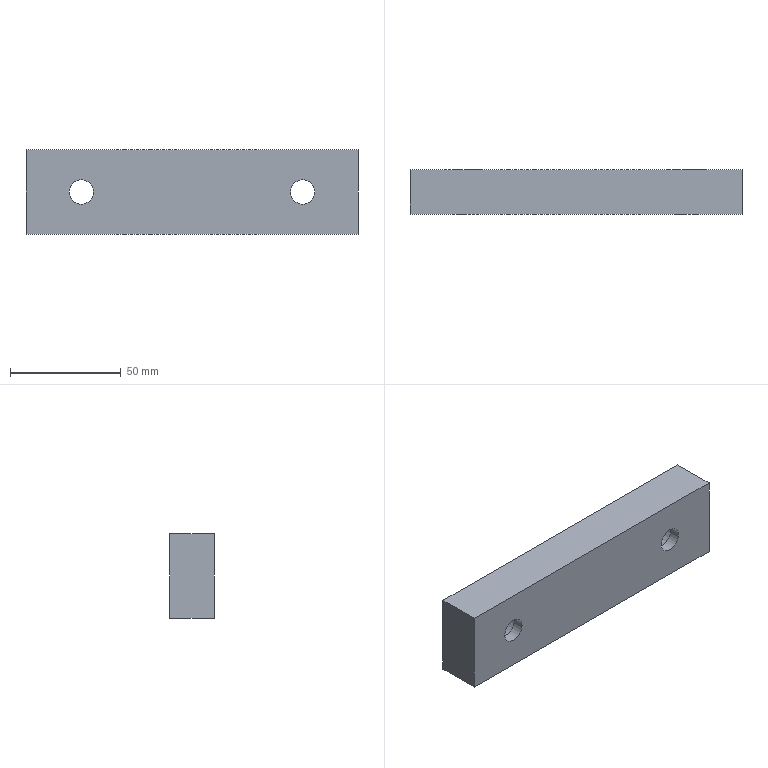Part | NX | features solid 2 | 1 solid | 12 faces | box 150 x 20 x 38 mm | volume 105834 mm3 | plane 8 | cylinder 4 | commonest cylinder face diameters 11 x2 17.5 x2
STEP:
#1=CARTESIAN_POINT('',(455.,825.,-87.));
#2=VERTEX_POINT('',#1);
#3=CARTESIAN_POINT('',(455.,805.,-87.));
#4=VERTEX_POINT('',#3);
#5=CARTESIAN_POINT('',(455.,815.,-87.));
#6=DIRECTION('',(0.,-1.,0.));
#7=VECTOR('',#6,1000.);
#8=LINE('',#5,#7);
#9=EDGE_CURVE('',#2,#4,#8,.T.);
#10=ORIENTED_EDGE('',*,*,#9,.T.);
#11=CARTESIAN_POINT('',(455.,805.,-125.));
#12=VERTEX_POINT('',#11);
#13=CARTESIAN_POINT('',(455.,805.,-106.));
#14=DIRECTION('',(0.,0.,-1.));
#15=VECTOR('',#14,1000.);
#16=LINE('',#13,#15);
#17=EDGE_CURVE('',#4,#12,#16,.T.);
#18=ORIENTED_EDGE('',*,*,#17,.T.);
#19=CARTESIAN_POINT('',(455.,825.,-125.));
#20=VERTEX_POINT('',#19);
#21=CARTESIAN_POINT('',(455.,815.,-125.));
#22=DIRECTION('',(0.,1.,0.));
#23=VECTOR('',#22,1000.);
#24=LINE('',#21,#23);
#25=EDGE_CURVE('',#12,#20,#24,.T.);
#26=ORIENTED_EDGE('',*,*,#25,.T.);
#27=CARTESIAN_POINT('',(455.,825.,-106.));
#28=DIRECTION('',(0.,0.,1.));
#29=VECTOR('',#28,1000.);
#30=LINE('',#27,#29);
#31=EDGE_CURVE('',#20,#2,#30,.T.);
#32=ORIENTED_EDGE('',*,*,#31,.T.);
#33=EDGE_LOOP('',(#10,#18,#26,#32));
#34=FACE_BOUND('',#33,.T.);
#35=CARTESIAN_POINT('',(455.,815.,-106.));
#36=DIRECTION('',(1.,0.,0.));
#37=DIRECTION('',(0.,1.,0.));
#38=AXIS2_PLACEMENT_3D('',#35,#36,#37);
#39=PLANE('',#38);
#40=ADVANCED_FACE('',(#34),#39,.T.);
#41=CARTESIAN_POINT('',(305.,825.,-87.));
#42=VERTEX_POINT('',#41);
#43=CARTESIAN_POINT('',(305.,825.,-87.));
#44=DIRECTION('',(1.,0.,0.));
#45=VECTOR('',#44,1000.);
#46=LINE('',#43,#45);
#47=EDGE_CURVE('',#42,#2,#46,.T.);
#48=ORIENTED_EDGE('',*,*,#47,.F.);
#49=CARTESIAN_POINT('',(305.,805.,-87.));
#50=VERTEX_POINT('',#49);
#51=CARTESIAN_POINT('',(305.,815.,-87.));
#52=DIRECTION('',(0.,1.,0.));
#53=VECTOR('',#52,1000.);
#54=LINE('',#51,#53);
#55=EDGE_CURVE('',#50,#42,#54,.T.);
#56=ORIENTED_EDGE('',*,*,#55,.F.);
#57=CARTESIAN_POINT('',(305.,805.,-87.));
#58=DIRECTION('',(1.,0.,0.));
#59=VECTOR('',#58,1000.);
#60=LINE('',#57,#59);
#61=EDGE_CURVE('',#50,#4,#60,.T.);
#62=ORIENTED_EDGE('',*,*,#61,.T.);
#63=ORIENTED_EDGE('',*,*,#9,.F.);
#64=EDGE_LOOP('',(#48,#56,#62,#63));
#65=FACE_BOUND('',#64,.T.);
#66=CARTESIAN_POINT('',(305.,815.,-87.));
#67=DIRECTION('',(0.,0.,1.));
#68=DIRECTION('',(-1.,0.,0.));
#69=AXIS2_PLACEMENT_3D('',#66,#67,#68);
#70=PLANE('',#69);
#71=ADVANCED_FACE('',(#65),#70,.T.);
#72=CARTESIAN_POINT('',(324.5,805.,-106.));
#73=VERTEX_POINT('',#72);
#74=CARTESIAN_POINT('',(330.,805.,-106.));
#75=DIRECTION('',(0.,-1.,0.));
#76=DIRECTION('',(-1.,0.,0.));
#77=AXIS2_PLACEMENT_3D('',#74,#75,#76);
#78=CIRCLE('',#77,5.5);
#79=EDGE_CURVE('',#73,#73,#78,.T.);
#80=ORIENTED_EDGE('',*,*,#79,.F.);
#81=EDGE_LOOP('',(#80));
#82=FACE_BOUND('',#81,.T.);
#83=CARTESIAN_POINT('',(424.5,805.,-106.));
#84=VERTEX_POINT('',#83);
#85=CARTESIAN_POINT('',(430.,805.,-106.));
#86=DIRECTION('',(0.,-1.,0.));
#87=DIRECTION('',(-1.,0.,0.));
#88=AXIS2_PLACEMENT_3D('',#85,#86,#87);
#89=CIRCLE('',#88,5.5);
#90=EDGE_CURVE('',#84,#84,#89,.T.);
#91=ORIENTED_EDGE('',*,*,#90,.F.);
#92=EDGE_LOOP('',(#91));
#93=FACE_BOUND('',#92,.T.);
#94=ORIENTED_EDGE('',*,*,#61,.F.);
#95=CARTESIAN_POINT('',(305.,805.,-125.));
#96=VERTEX_POINT('',#95);
#97=CARTESIAN_POINT('',(305.,805.,-106.));
#98=DIRECTION('',(0.,0.,1.));
#99=VECTOR('',#98,1000.);
#100=LINE('',#97,#99);
#101=EDGE_CURVE('',#96,#50,#100,.T.);
#102=ORIENTED_EDGE('',*,*,#101,.F.);
#103=CARTESIAN_POINT('',(305.,805.,-125.));
#104=DIRECTION('',(1.,0.,0.));
#105=VECTOR('',#104,1000.);
#106=LINE('',#103,#105);
#107=EDGE_CURVE('',#96,#12,#106,.T.);
#108=ORIENTED_EDGE('',*,*,#107,.T.);
#109=ORIENTED_EDGE('',*,*,#17,.F.);
#110=EDGE_LOOP('',(#94,#102,#108,#109));
#111=FACE_BOUND('',#110,.T.);
#112=CARTESIAN_POINT('',(305.,805.,-106.));
#113=DIRECTION('',(0.,-1.,0.));
#114=DIRECTION('',(1.,0.,0.));
#115=AXIS2_PLACEMENT_3D('',#112,#113,#114);
#116=PLANE('',#115);
#117=ADVANCED_FACE('',(#82,#93,#111),#116,.T.);
#118=ORIENTED_EDGE('',*,*,#107,.F.);
#119=CARTESIAN_POINT('',(305.,825.,-125.));
#120=VERTEX_POINT('',#119);
#121=CARTESIAN_POINT('',(305.,815.,-125.));
#122=DIRECTION('',(0.,-1.,0.));
#123=VECTOR('',#122,1000.);
#124=LINE('',#121,#123);
#125=EDGE_CURVE('',#120,#96,#124,.T.);
#126=ORIENTED_EDGE('',*,*,#125,.F.);
#127=CARTESIAN_POINT('',(305.,825.,-125.));
#128=DIRECTION('',(1.,0.,0.));
#129=VECTOR('',#128,1000.);
#130=LINE('',#127,#129);
#131=EDGE_CURVE('',#120,#20,#130,.T.);
#132=ORIENTED_EDGE('',*,*,#131,.T.);
#133=ORIENTED_EDGE('',*,*,#25,.F.);
#134=EDGE_LOOP('',(#118,#126,#132,#133));
#135=FACE_BOUND('',#134,.T.);
#136=CARTESIAN_POINT('',(305.,815.,-125.));
#137=DIRECTION('',(0.,0.,-1.));
#138=DIRECTION('',(1.,0.,0.));
#139=AXIS2_PLACEMENT_3D('',#136,#137,#138);
#140=PLANE('',#139);
#141=ADVANCED_FACE('',(#135),#140,.T.);
#142=CARTESIAN_POINT('',(305.,825.,-106.));
#143=DIRECTION('',(0.,0.,-1.));
#144=VECTOR('',#143,1000.);
#145=LINE('',#142,#144);
#146=EDGE_CURVE('',#42,#120,#145,.T.);
#147=ORIENTED_EDGE('',*,*,#146,.T.);
#148=ORIENTED_EDGE('',*,*,#125,.T.);
#149=ORIENTED_EDGE('',*,*,#101,.T.);
#150=ORIENTED_EDGE('',*,*,#55,.T.);
#151=EDGE_LOOP('',(#147,#148,#149,#150));
#152=FACE_BOUND('',#151,.T.);
#153=CARTESIAN_POINT('',(305.,815.,-106.));
#154=DIRECTION('',(-1.,0.,0.));
#155=DIRECTION('',(0.,-1.,0.));
#156=AXIS2_PLACEMENT_3D('',#153,#154,#155);
#157=PLANE('',#156);
#158=ADVANCED_FACE('',(#152),#157,.T.);
#159=CARTESIAN_POINT('',(338.75,825.,-106.));
#160=VERTEX_POINT('',#159);
#161=CARTESIAN_POINT('',(330.,825.,-106.));
#162=DIRECTION('',(0.,1.,0.));
#163=DIRECTION('',(1.,0.,0.));
#164=AXIS2_PLACEMENT_3D('',#161,#162,#163);
#165=CIRCLE('',#164,8.75);
#166=EDGE_CURVE('',#160,#160,#165,.T.);
#167=ORIENTED_EDGE('',*,*,#166,.F.);
#168=EDGE_LOOP('',(#167));
#169=FACE_BOUND('',#168,.T.);
#170=CARTESIAN_POINT('',(438.75,825.,-106.));
#171=VERTEX_POINT('',#170);
#172=CARTESIAN_POINT('',(430.,825.,-106.));
#173=DIRECTION('',(0.,1.,0.));
#174=DIRECTION('',(1.,0.,0.));
#175=AXIS2_PLACEMENT_3D('',#172,#173,#174);
#176=CIRCLE('',#175,8.75);
#177=EDGE_CURVE('',#171,#171,#176,.T.);
#178=ORIENTED_EDGE('',*,*,#177,.F.);
#179=EDGE_LOOP('',(#178));
#180=FACE_BOUND('',#179,.T.);
#181=ORIENTED_EDGE('',*,*,#146,.F.);
#182=ORIENTED_EDGE('',*,*,#47,.T.);
#183=ORIENTED_EDGE('',*,*,#31,.F.);
#184=ORIENTED_EDGE('',*,*,#131,.F.);
#185=EDGE_LOOP('',(#181,#182,#183,#184));
#186=FACE_BOUND('',#185,.T.);
#187=CARTESIAN_POINT('',(305.,825.,-106.));
#188=DIRECTION('',(0.,1.,0.));
#189=DIRECTION('',(-1.,0.,0.));
#190=AXIS2_PLACEMENT_3D('',#187,#188,#189);
#191=PLANE('',#190);
#192=ADVANCED_FACE('',(#169,#180,#186),#191,.T.);
#193=CARTESIAN_POINT('',(435.5,810.,-106.));
#194=VERTEX_POINT('',#193);
#195=CARTESIAN_POINT('',(430.,810.,-106.));
#196=DIRECTION('',(0.,1.,0.));
#197=DIRECTION('',(1.,0.,0.));
#198=AXIS2_PLACEMENT_3D('',#195,#196,#197);
#199=CIRCLE('',#198,5.5);
#200=EDGE_CURVE('',#194,#194,#199,.F.);
#201=ORIENTED_EDGE('',*,*,#200,.F.);
#202=EDGE_LOOP('',(#201));
#203=FACE_BOUND('',#202,.T.);
#204=ORIENTED_EDGE('',*,*,#90,.T.);
#205=EDGE_LOOP('',(#204));
#206=FACE_BOUND('',#205,.T.);
#207=CARTESIAN_POINT('',(430.,805.,-106.));
#208=DIRECTION('',(0.,1.,0.));
#209=DIRECTION('',(-1.,0.,0.));
#210=AXIS2_PLACEMENT_3D('',#207,#208,#209);
#211=CYLINDRICAL_SURFACE('',#210,5.5);
#212=ADVANCED_FACE('',(#203,#206),#211,.F.);
#213=CARTESIAN_POINT('',(421.25,810.,-106.));
#214=VERTEX_POINT('',#213);
#215=CARTESIAN_POINT('',(430.,810.,-106.));
#216=DIRECTION('',(0.,-1.,0.));
#217=DIRECTION('',(-1.,0.,0.));
#218=AXIS2_PLACEMENT_3D('',#215,#216,#217);
#219=CIRCLE('',#218,8.75);
#220=EDGE_CURVE('',#214,#214,#219,.T.);
#221=ORIENTED_EDGE('',*,*,#220,.F.);
#222=EDGE_LOOP('',(#221));
#223=FACE_BOUND('',#222,.T.);
#224=ORIENTED_EDGE('',*,*,#200,.T.);
#225=EDGE_LOOP('',(#224));
#226=FACE_BOUND('',#225,.T.);
#227=CARTESIAN_POINT('',(430.,810.,-106.));
#228=DIRECTION('',(0.,-1.,0.));
#229=DIRECTION('',(1.,0.,0.));
#230=AXIS2_PLACEMENT_3D('',#227,#228,#229);
#231=PLANE('',#230);
#232=ADVANCED_FACE('',(#223,#226),#231,.F.);
#233=ORIENTED_EDGE('',*,*,#177,.T.);
#234=EDGE_LOOP('',(#233));
#235=FACE_BOUND('',#234,.T.);
#236=ORIENTED_EDGE('',*,*,#220,.T.);
#237=EDGE_LOOP('',(#236));
#238=FACE_BOUND('',#237,.T.);
#239=CARTESIAN_POINT('',(430.,810.,-106.));
#240=DIRECTION('',(0.,1.,0.));
#241=DIRECTION('',(-1.,0.,0.));
#242=AXIS2_PLACEMENT_3D('',#239,#240,#241);
#243=CYLINDRICAL_SURFACE('',#242,8.75);
#244=ADVANCED_FACE('',(#235,#238),#243,.F.);
#245=CARTESIAN_POINT('',(335.5,810.,-106.));
#246=VERTEX_POINT('',#245);
#247=CARTESIAN_POINT('',(330.,810.,-106.));
#248=DIRECTION('',(0.,1.,0.));
#249=DIRECTION('',(1.,0.,0.));
#250=AXIS2_PLACEMENT_3D('',#247,#248,#249);
#251=CIRCLE('',#250,5.5);
#252=EDGE_CURVE('',#246,#246,#251,.F.);
#253=ORIENTED_EDGE('',*,*,#252,.F.);
#254=EDGE_LOOP('',(#253));
#255=FACE_BOUND('',#254,.T.);
#256=ORIENTED_EDGE('',*,*,#79,.T.);
#257=EDGE_LOOP('',(#256));
#258=FACE_BOUND('',#257,.T.);
#259=CARTESIAN_POINT('',(330.,805.,-106.));
#260=DIRECTION('',(0.,1.,0.));
#261=DIRECTION('',(-1.,0.,0.));
#262=AXIS2_PLACEMENT_3D('',#259,#260,#261);
#263=CYLINDRICAL_SURFACE('',#262,5.5);
#264=ADVANCED_FACE('',(#255,#258),#263,.F.);
#265=CARTESIAN_POINT('',(321.25,810.,-106.));
#266=VERTEX_POINT('',#265);
#267=CARTESIAN_POINT('',(330.,810.,-106.));
#268=DIRECTION('',(0.,-1.,0.));
#269=DIRECTION('',(-1.,0.,0.));
#270=AXIS2_PLACEMENT_3D('',#267,#268,#269);
#271=CIRCLE('',#270,8.75);
#272=EDGE_CURVE('',#266,#266,#271,.T.);
#273=ORIENTED_EDGE('',*,*,#272,.F.);
#274=EDGE_LOOP('',(#273));
#275=FACE_BOUND('',#274,.T.);
#276=ORIENTED_EDGE('',*,*,#252,.T.);
#277=EDGE_LOOP('',(#276));
#278=FACE_BOUND('',#277,.T.);
#279=CARTESIAN_POINT('',(330.,810.,-106.));
#280=DIRECTION('',(0.,-1.,0.));
#281=DIRECTION('',(1.,0.,0.));
#282=AXIS2_PLACEMENT_3D('',#279,#280,#281);
#283=PLANE('',#282);
#284=ADVANCED_FACE('',(#275,#278),#283,.F.);
#285=ORIENTED_EDGE('',*,*,#166,.T.);
#286=EDGE_LOOP('',(#285));
#287=FACE_BOUND('',#286,.T.);
#288=ORIENTED_EDGE('',*,*,#272,.T.);
#289=EDGE_LOOP('',(#288));
#290=FACE_BOUND('',#289,.T.);
#291=CARTESIAN_POINT('',(330.,810.,-106.));
#292=DIRECTION('',(0.,1.,0.));
#293=DIRECTION('',(-1.,0.,0.));
#294=AXIS2_PLACEMENT_3D('',#291,#292,#293);
#295=CYLINDRICAL_SURFACE('',#294,8.75);
#296=ADVANCED_FACE('',(#287,#290),#295,.F.);
#297=CLOSED_SHELL('',(#40,#71,#117,#141,#158,#192,#212,#232,#244,#264,#284,#296));
#298=MANIFOLD_SOLID_BREP('',#297);
#299=(LENGTH_UNIT()NAMED_UNIT(*)SI_UNIT(.MILLI.,.METRE.));
#300=UNCERTAINTY_MEASURE_WITH_UNIT(LENGTH_MEASURE(0.00001),#299,'','');
#301=(NAMED_UNIT(*)PLANE_ANGLE_UNIT()SI_UNIT($,.RADIAN.));
#302=(NAMED_UNIT(*)SI_UNIT($,.STERADIAN.)SOLID_ANGLE_UNIT());
#303=(GEOMETRIC_REPRESENTATION_CONTEXT(3)GLOBAL_UNCERTAINTY_ASSIGNED_CONTEXT((#300))GLOBAL_UNIT_ASSIGNED_CONTEXT((#299,#301,#302))REPRESENTATION_CONTEXT('',''));
#304=ADVANCED_BREP_SHAPE_REPRESENTATION('',(#298),#303);